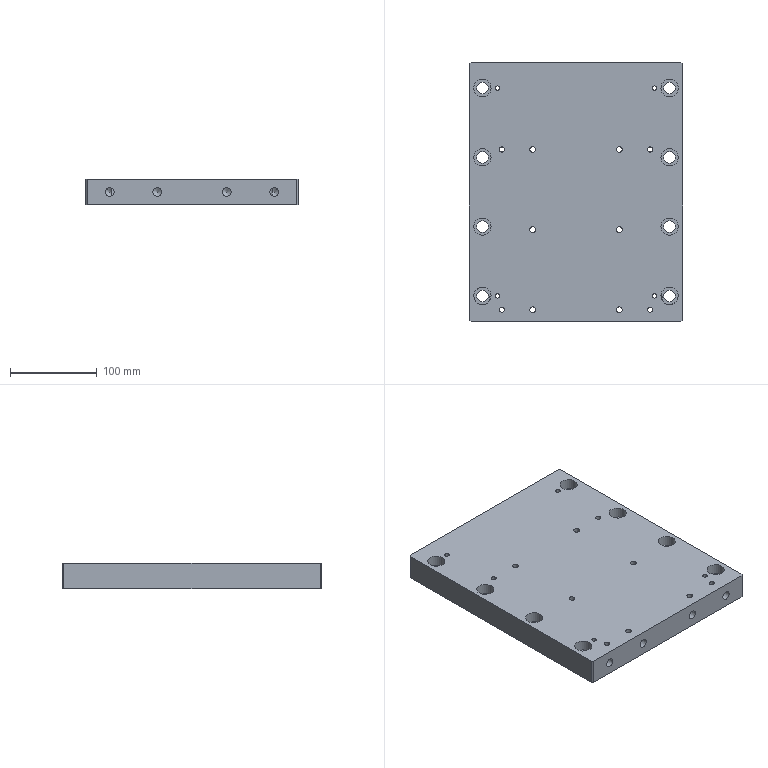Part | 1 solid | 56 faces | box 246 x 300 x 30 mm | volume 2140073 mm3 | cylinder 34 | plane 18 | cone 4 | commonest cylinder face diameters 13.5 x8 20 x8 6.8 x6 5 x4 6 x4 10.2 x4